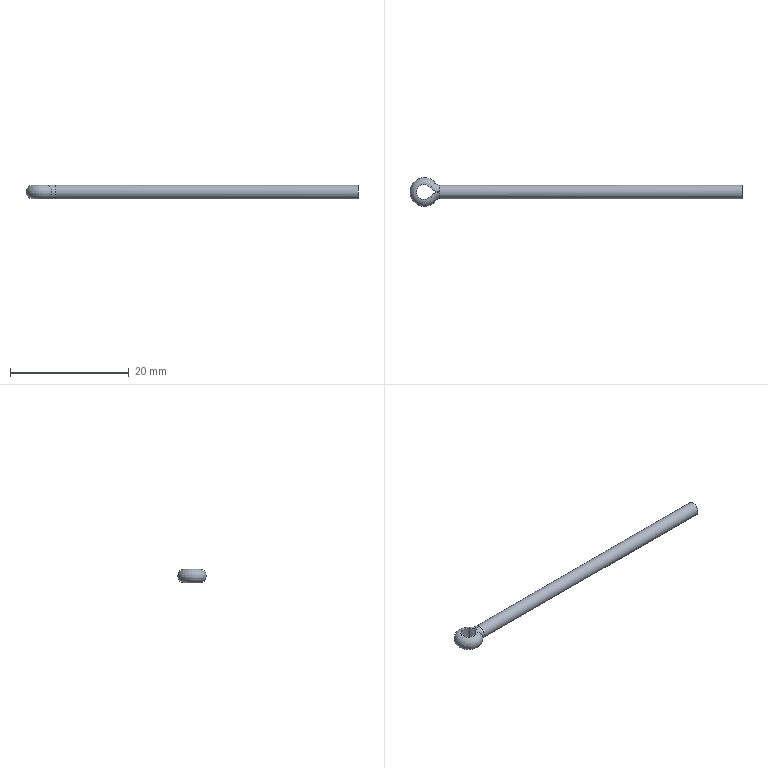Part | NX | features solid 2 | 1 solid | 8 faces | box 55.816 x 4.826 x 2.286 mm | volume 232.12 mm3 | cylinder 4 | torus 3 | plane 1 | commonest cylinder face diameters 4.064 x2 2.286 x1 2.54 x1
STEP:
#1=CARTESIAN_POINT('',(-52.402,-0.7815,-1.143));
#2=VERTEX_POINT('',#1);
#3=CARTESIAN_POINT('',(-52.402,-0.7815,1.143));
#4=VERTEX_POINT('',#3);
#5=CARTESIAN_POINT('',(-52.402,-0.7815,-1.143));
#6=DIRECTION('',(0.,0.,1.));
#7=VECTOR('',#6,1000.);
#8=LINE('',#5,#7);
#9=EDGE_CURVE('',#2,#4,#8,.T.);
#10=ORIENTED_EDGE('',*,*,#9,.F.);
#11=CARTESIAN_POINT('',(-52.402,0.7815,-1.143));
#12=VERTEX_POINT('',#11);
#13=CARTESIAN_POINT('',(-53.403,0.,-1.143));
#14=DIRECTION('',(0.,0.,-1.));
#15=DIRECTION('',(-1.,0.,0.));
#16=AXIS2_PLACEMENT_3D('',#13,#14,#15);
#17=CIRCLE('',#16,1.27);
#18=EDGE_CURVE('',#12,#2,#17,.F.);
#19=ORIENTED_EDGE('',*,*,#18,.F.);
#20=CARTESIAN_POINT('',(-52.402,0.7815,1.143));
#21=VERTEX_POINT('',#20);
#22=CARTESIAN_POINT('',(-52.402,0.7815,-1.143));
#23=DIRECTION('',(0.,0.,1.));
#24=VECTOR('',#23,1000.);
#25=LINE('',#22,#24);
#26=EDGE_CURVE('',#12,#21,#25,.T.);
#27=ORIENTED_EDGE('',*,*,#26,.T.);
#28=CARTESIAN_POINT('',(-53.403,0.,1.143));
#29=DIRECTION('',(0.,0.,-1.));
#30=DIRECTION('',(-1.,0.,0.));
#31=AXIS2_PLACEMENT_3D('',#28,#29,#30);
#32=CIRCLE('',#31,1.27);
#33=EDGE_CURVE('',#4,#21,#32,.T.);
#34=ORIENTED_EDGE('',*,*,#33,.F.);
#35=EDGE_LOOP('',(#10,#19,#27,#34));
#36=FACE_BOUND('',#35,.T.);
#37=CARTESIAN_POINT('',(-53.403,0.,0.));
#38=DIRECTION('',(0.,0.,-1.));
#39=DIRECTION('',(-1.,0.,0.));
#40=AXIS2_PLACEMENT_3D('',#37,#38,#39);
#41=CYLINDRICAL_SURFACE('',#40,1.27);
#42=ADVANCED_FACE('',(#36),#41,.F.);
#43=CARTESIAN_POINT('',(-52.402,-0.7815,0.));
#44=DIRECTION('',(0.6154,0.7882,0.));
#45=DIRECTION('',(-0.7882,0.6154,0.));
#46=AXIS2_PLACEMENT_3D('',#43,#44,#45);
#47=CIRCLE('',#46,1.143);
#48=EDGE_CURVE('',#4,#2,#47,.T.);
#49=ORIENTED_EDGE('',*,*,#48,.F.);
#50=ORIENTED_EDGE('',*,*,#33,.T.);
#51=CARTESIAN_POINT('',(-52.402,0.7815,0.));
#52=DIRECTION('',(-0.6154,0.7882,0.));
#53=DIRECTION('',(-0.7882,-0.6154,0.));
#54=AXIS2_PLACEMENT_3D('',#51,#52,#53);
#55=CIRCLE('',#54,1.143);
#56=EDGE_CURVE('',#21,#12,#55,.T.);
#57=ORIENTED_EDGE('',*,*,#56,.T.);
#58=ORIENTED_EDGE('',*,*,#18,.T.);
#59=EDGE_LOOP('',(#49,#50,#57,#58));
#60=FACE_BOUND('',#59,.T.);
#61=CARTESIAN_POINT('',(-53.403,0.,0.));
#62=DIRECTION('',(0.,0.,-1.));
#63=DIRECTION('',(-1.,0.,0.));
#64=AXIS2_PLACEMENT_3D('',#61,#62,#63);
#65=TOROIDAL_SURFACE('',#64,1.27,1.143);
#66=ADVANCED_FACE('',(#60),#65,.T.);
#67=CARTESIAN_POINT('',(-50.8,0.,-1.143));
#68=VERTEX_POINT('',#67);
#69=CARTESIAN_POINT('',(-50.8,0.,1.143));
#70=VERTEX_POINT('',#69);
#71=CARTESIAN_POINT('',(-50.8,0.,-1.143));
#72=DIRECTION('',(0.,0.,1.));
#73=VECTOR('',#72,1000.);
#74=LINE('',#71,#73);
#75=EDGE_CURVE('',#68,#70,#74,.T.);
#76=ORIENTED_EDGE('',*,*,#75,.F.);
#77=CARTESIAN_POINT('',(-50.8,-2.032,-1.143));
#78=DIRECTION('',(0.,0.,1.));
#79=DIRECTION('',(1.,0.,0.));
#80=AXIS2_PLACEMENT_3D('',#77,#78,#79);
#81=CIRCLE('',#80,2.032);
#82=EDGE_CURVE('',#2,#68,#81,.F.);
#83=ORIENTED_EDGE('',*,*,#82,.F.);
#84=ORIENTED_EDGE('',*,*,#9,.T.);
#85=CARTESIAN_POINT('',(-50.8,-2.032,1.143));
#86=DIRECTION('',(0.,0.,1.));
#87=DIRECTION('',(1.,0.,0.));
#88=AXIS2_PLACEMENT_3D('',#85,#86,#87);
#89=CIRCLE('',#88,2.032);
#90=EDGE_CURVE('',#70,#4,#89,.T.);
#91=ORIENTED_EDGE('',*,*,#90,.F.);
#92=EDGE_LOOP('',(#76,#83,#84,#91));
#93=FACE_BOUND('',#92,.T.);
#94=CARTESIAN_POINT('',(-50.8,-2.032,0.));
#95=DIRECTION('',(0.,0.,1.));
#96=DIRECTION('',(1.,0.,0.));
#97=AXIS2_PLACEMENT_3D('',#94,#95,#96);
#98=CYLINDRICAL_SURFACE('',#97,2.032);
#99=ADVANCED_FACE('',(#93),#98,.T.);
#100=CARTESIAN_POINT('',(-50.8,0.,0.));
#101=DIRECTION('',(1.,0.,0.));
#102=DIRECTION('',(0.,1.,0.));
#103=AXIS2_PLACEMENT_3D('',#100,#101,#102);
#104=CIRCLE('',#103,1.143);
#105=EDGE_CURVE('',#70,#68,#104,.T.);
#106=ORIENTED_EDGE('',*,*,#105,.F.);
#107=ORIENTED_EDGE('',*,*,#90,.T.);
#108=ORIENTED_EDGE('',*,*,#48,.T.);
#109=ORIENTED_EDGE('',*,*,#82,.T.);
#110=EDGE_LOOP('',(#106,#107,#108,#109));
#111=FACE_BOUND('',#110,.T.);
#112=CARTESIAN_POINT('',(-50.8,-2.032,0.));
#113=DIRECTION('',(0.,0.,1.));
#114=DIRECTION('',(1.,0.,0.));
#115=AXIS2_PLACEMENT_3D('',#112,#113,#114);
#116=TOROIDAL_SURFACE('',#115,2.032,1.143);
#117=ADVANCED_FACE('',(#111),#116,.T.);
#118=CARTESIAN_POINT('',(0.,1.143,0.));
#119=VERTEX_POINT('',#118);
#120=CARTESIAN_POINT('',(0.,0.,0.));
#121=DIRECTION('',(1.,0.,0.));
#122=DIRECTION('',(0.,1.,0.));
#123=AXIS2_PLACEMENT_3D('',#120,#121,#122);
#124=CIRCLE('',#123,1.143);
#125=EDGE_CURVE('',#119,#119,#124,.T.);
#126=ORIENTED_EDGE('',*,*,#125,.F.);
#127=EDGE_LOOP('',(#126));
#128=FACE_BOUND('',#127,.T.);
#129=CARTESIAN_POINT('',(-50.8,0.,0.));
#130=DIRECTION('',(-1.,0.,0.));
#131=DIRECTION('',(0.,-1.,0.));
#132=AXIS2_PLACEMENT_3D('',#129,#130,#131);
#133=CIRCLE('',#132,1.143);
#134=EDGE_CURVE('',#68,#70,#133,.F.);
#135=ORIENTED_EDGE('',*,*,#134,.T.);
#136=ORIENTED_EDGE('',*,*,#105,.T.);
#137=EDGE_LOOP('',(#135,#136));
#138=FACE_BOUND('',#137,.T.);
#139=CARTESIAN_POINT('',(-50.8,0.,0.));
#140=DIRECTION('',(1.,0.,0.));
#141=DIRECTION('',(0.,0.,-1.));
#142=AXIS2_PLACEMENT_3D('',#139,#140,#141);
#143=CYLINDRICAL_SURFACE('',#142,1.143);
#144=ADVANCED_FACE('',(#128,#138),#143,.T.);
#145=ORIENTED_EDGE('',*,*,#125,.T.);
#146=EDGE_LOOP('',(#145));
#147=FACE_BOUND('',#146,.T.);
#148=CARTESIAN_POINT('',(0.,0.,0.));
#149=DIRECTION('',(1.,0.,0.));
#150=DIRECTION('',(0.,0.,-1.));
#151=AXIS2_PLACEMENT_3D('',#148,#149,#150);
#152=PLANE('',#151);
#153=ADVANCED_FACE('',(#147),#152,.T.);
#154=ORIENTED_EDGE('',*,*,#75,.T.);
#155=CARTESIAN_POINT('',(-50.8,2.032,1.143));
#156=DIRECTION('',(0.,0.,-1.));
#157=DIRECTION('',(1.,0.,0.));
#158=AXIS2_PLACEMENT_3D('',#155,#156,#157);
#159=CIRCLE('',#158,2.032);
#160=EDGE_CURVE('',#70,#21,#159,.T.);
#161=ORIENTED_EDGE('',*,*,#160,.T.);
#162=ORIENTED_EDGE('',*,*,#26,.F.);
#163=CARTESIAN_POINT('',(-50.8,2.032,-1.143));
#164=DIRECTION('',(0.,0.,-1.));
#165=DIRECTION('',(1.,0.,0.));
#166=AXIS2_PLACEMENT_3D('',#163,#164,#165);
#167=CIRCLE('',#166,2.032);
#168=EDGE_CURVE('',#12,#68,#167,.F.);
#169=ORIENTED_EDGE('',*,*,#168,.T.);
#170=EDGE_LOOP('',(#154,#161,#162,#169));
#171=FACE_BOUND('',#170,.T.);
#172=CARTESIAN_POINT('',(-50.8,2.032,0.));
#173=DIRECTION('',(0.,0.,1.));
#174=DIRECTION('',(1.,0.,0.));
#175=AXIS2_PLACEMENT_3D('',#172,#173,#174);
#176=CYLINDRICAL_SURFACE('',#175,2.032);
#177=ADVANCED_FACE('',(#171),#176,.T.);
#178=ORIENTED_EDGE('',*,*,#134,.F.);
#179=ORIENTED_EDGE('',*,*,#168,.F.);
#180=ORIENTED_EDGE('',*,*,#56,.F.);
#181=ORIENTED_EDGE('',*,*,#160,.F.);
#182=EDGE_LOOP('',(#178,#179,#180,#181));
#183=FACE_BOUND('',#182,.T.);
#184=CARTESIAN_POINT('',(-50.8,2.032,0.));
#185=DIRECTION('',(0.,0.,1.));
#186=DIRECTION('',(1.,0.,0.));
#187=AXIS2_PLACEMENT_3D('',#184,#185,#186);
#188=TOROIDAL_SURFACE('',#187,2.032,1.143);
#189=ADVANCED_FACE('',(#183),#188,.T.);
#190=CLOSED_SHELL('',(#42,#66,#99,#117,#144,#153,#177,#189));
#191=MANIFOLD_SOLID_BREP('',#190);
#192=(LENGTH_UNIT()NAMED_UNIT(*)SI_UNIT(.MILLI.,.METRE.));
#193=UNCERTAINTY_MEASURE_WITH_UNIT(LENGTH_MEASURE(0.00001),#192,'','');
#194=(NAMED_UNIT(*)PLANE_ANGLE_UNIT()SI_UNIT($,.RADIAN.));
#195=(NAMED_UNIT(*)SI_UNIT($,.STERADIAN.)SOLID_ANGLE_UNIT());
#196=(GEOMETRIC_REPRESENTATION_CONTEXT(3)GLOBAL_UNCERTAINTY_ASSIGNED_CONTEXT((#193))GLOBAL_UNIT_ASSIGNED_CONTEXT((#192,#194,#195))REPRESENTATION_CONTEXT('',''));
#197=ADVANCED_BREP_SHAPE_REPRESENTATION('',(#191),#196);